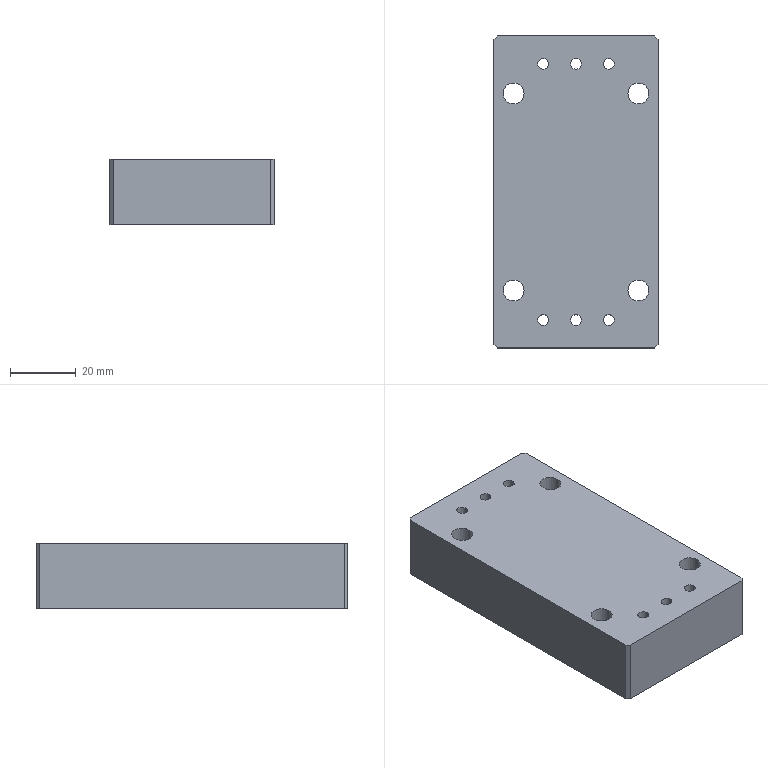Part | SolidWorks | features HoleWzd 2, Chamfer 1, Extrusion 1 | 1 solid | 54 faces | box 50 x 95 x 20 mm | volume 89595 mm3 | cylinder 28 | plane 14 | cone 12 | commonest cylinder face diameters 3.3 x12 6.4 x8 11 x8